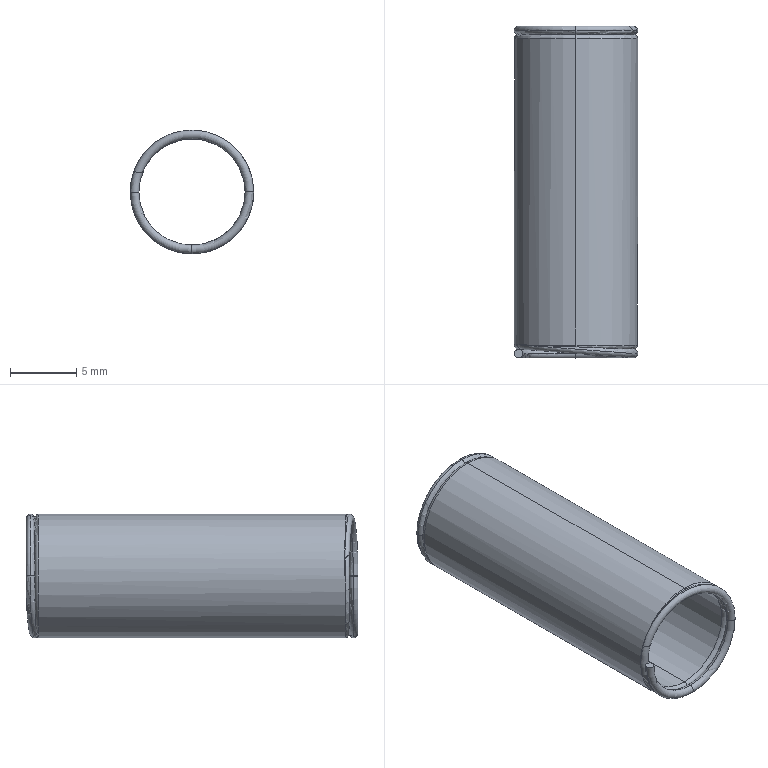Part | STEP file | C-VUR8-25 | 1 solid | 32 faces | box 9.3 x 25 x 9.325 mm | volume 430.371 mm3 | torus 26 | cylinder 4 | plane 2 | commonest cylinder face diameters 8 x2 9.3 x2
STEP:
#1=CARTESIAN_POINT('',(0.,-12.175,-4.65));
#2=VERTEX_POINT('',#1);
#3=CARTESIAN_POINT('',(0.,-12.175,-4.));
#4=VERTEX_POINT('',#3);
#5=CARTESIAN_POINT('',(0.,-12.175,-4.325));
#6=DIRECTION('',(-1.,0.,0.));
#7=DIRECTION('',(0.,0.,1.));
#8=AXIS2_PLACEMENT_3D('',#5,#6,#7);
#9=CIRCLE('',#8,0.325);
#10=EDGE_CURVE('',#2,#4,#9,.T.);
#11=ORIENTED_EDGE('',*,*,#10,.F.);
#12=CARTESIAN_POINT('',(4.65,-12.175,0.));
#13=VERTEX_POINT('',#12);
#14=CARTESIAN_POINT('',(0.,-12.175,0.));
#15=DIRECTION('',(0.,-1.,0.));
#16=DIRECTION('',(0.,0.,-1.));
#17=AXIS2_PLACEMENT_3D('',#14,#15,#16);
#18=CIRCLE('',#17,4.65);
#19=EDGE_CURVE('',#2,#13,#18,.T.);
#20=ORIENTED_EDGE('',*,*,#19,.T.);
#21=CARTESIAN_POINT('',(4.649,-12.2,0.));
#22=VERTEX_POINT('',#21);
#23=CARTESIAN_POINT('',(4.325,-12.175,0.));
#24=DIRECTION('',(0.,0.,1.));
#25=DIRECTION('',(1.,0.,0.));
#26=AXIS2_PLACEMENT_3D('',#23,#24,#25);
#27=CIRCLE('',#26,0.325);
#28=EDGE_CURVE('',#22,#13,#27,.T.);
#29=ORIENTED_EDGE('',*,*,#28,.F.);
#30=CARTESIAN_POINT('',(4.,-12.175,0.));
#31=VERTEX_POINT('',#30);
#32=CARTESIAN_POINT('',(4.325,-12.175,0.));
#33=DIRECTION('',(0.,0.,1.));
#34=DIRECTION('',(1.,0.,0.));
#35=AXIS2_PLACEMENT_3D('',#32,#33,#34);
#36=CIRCLE('',#35,0.325);
#37=EDGE_CURVE('',#31,#22,#36,.T.);
#38=ORIENTED_EDGE('',*,*,#37,.F.);
#39=CARTESIAN_POINT('',(0.,-12.175,0.));
#40=DIRECTION('',(0.,-1.,0.));
#41=DIRECTION('',(0.,0.,-1.));
#42=AXIS2_PLACEMENT_3D('',#39,#40,#41);
#43=CIRCLE('',#42,4.);
#44=EDGE_CURVE('',#4,#31,#43,.T.);
#45=ORIENTED_EDGE('',*,*,#44,.F.);
#46=EDGE_LOOP('',(#11,#20,#29,#38,#45));
#47=FACE_OUTER_BOUND('',#46,.T.);
#48=CARTESIAN_POINT('',(0.,-12.175,0.));
#49=DIRECTION('',(0.,-1.,0.));
#50=DIRECTION('',(0.,0.,-1.));
#51=AXIS2_PLACEMENT_3D('',#48,#49,#50);
#52=TOROIDAL_SURFACE('',#51,4.325,0.325);
#53=ADVANCED_FACE('',(#47),#52,.T.);
#54=CARTESIAN_POINT('',(0.,-11.855,-4.268));
#55=VERTEX_POINT('',#54);
#56=CARTESIAN_POINT('',(0.,-12.175,-4.325));
#57=DIRECTION('',(-1.,0.,0.));
#58=DIRECTION('',(0.,0.,1.));
#59=AXIS2_PLACEMENT_3D('',#56,#57,#58);
#60=CIRCLE('',#59,0.325);
#61=EDGE_CURVE('',#4,#55,#60,.T.);
#62=ORIENTED_EDGE('',*,*,#61,.F.);
#63=ORIENTED_EDGE('',*,*,#44,.T.);
#64=CARTESIAN_POINT('',(4.001,-12.15,0.));
#65=VERTEX_POINT('',#64);
#66=CARTESIAN_POINT('',(4.325,-12.175,0.));
#67=DIRECTION('',(0.,0.,1.));
#68=DIRECTION('',(1.,0.,0.));
#69=AXIS2_PLACEMENT_3D('',#66,#67,#68);
#70=CIRCLE('',#69,0.325);
#71=EDGE_CURVE('',#65,#31,#70,.T.);
#72=ORIENTED_EDGE('',*,*,#71,.F.);
#73=CARTESIAN_POINT('',(4.268,-11.855,0.));
#74=VERTEX_POINT('',#73);
#75=CARTESIAN_POINT('',(4.325,-12.175,0.));
#76=DIRECTION('',(0.,0.,1.));
#77=DIRECTION('',(1.,0.,0.));
#78=AXIS2_PLACEMENT_3D('',#75,#76,#77);
#79=CIRCLE('',#78,0.325);
#80=EDGE_CURVE('',#74,#65,#79,.T.);
#81=ORIENTED_EDGE('',*,*,#80,.F.);
#82=CARTESIAN_POINT('',(0.,-11.855,0.));
#83=DIRECTION('',(0.,1.,0.));
#84=DIRECTION('',(0.,0.,1.));
#85=AXIS2_PLACEMENT_3D('',#82,#83,#84);
#86=CIRCLE('',#85,4.268);
#87=EDGE_CURVE('',#74,#55,#86,.T.);
#88=ORIENTED_EDGE('',*,*,#87,.T.);
#89=EDGE_LOOP('',(#62,#63,#72,#81,#88));
#90=FACE_OUTER_BOUND('',#89,.T.);
#91=CARTESIAN_POINT('',(0.,-12.175,0.));
#92=DIRECTION('',(0.,-1.,0.));
#93=DIRECTION('',(0.,0.,-1.));
#94=AXIS2_PLACEMENT_3D('',#91,#92,#93);
#95=TOROIDAL_SURFACE('',#94,4.325,0.325);
#96=ADVANCED_FACE('',(#90),#95,.T.);
#97=CARTESIAN_POINT('',(0.,12.175,4.65));
#98=VERTEX_POINT('',#97);
#99=CARTESIAN_POINT('',(0.,12.175,4.));
#100=VERTEX_POINT('',#99);
#101=CARTESIAN_POINT('',(0.,12.175,4.325));
#102=DIRECTION('',(-1.,0.,0.));
#103=DIRECTION('',(0.,0.,1.));
#104=AXIS2_PLACEMENT_3D('',#101,#102,#103);
#105=CIRCLE('',#104,0.325);
#106=EDGE_CURVE('',#98,#100,#105,.T.);
#107=ORIENTED_EDGE('',*,*,#106,.F.);
#108=CARTESIAN_POINT('',(4.65,12.175,0.));
#109=VERTEX_POINT('',#108);
#110=CARTESIAN_POINT('',(0.,12.175,0.));
#111=DIRECTION('',(0.,1.,0.));
#112=DIRECTION('',(0.,0.,1.));
#113=AXIS2_PLACEMENT_3D('',#110,#111,#112);
#114=CIRCLE('',#113,4.65);
#115=EDGE_CURVE('',#98,#109,#114,.T.);
#116=ORIENTED_EDGE('',*,*,#115,.T.);
#117=CARTESIAN_POINT('',(4.,12.175,0.));
#118=VERTEX_POINT('',#117);
#119=CARTESIAN_POINT('',(4.325,12.175,0.));
#120=DIRECTION('',(0.,0.,-1.));
#121=DIRECTION('',(-1.,0.,0.));
#122=AXIS2_PLACEMENT_3D('',#119,#120,#121);
#123=CIRCLE('',#122,0.325);
#124=EDGE_CURVE('',#118,#109,#123,.T.);
#125=ORIENTED_EDGE('',*,*,#124,.F.);
#126=CARTESIAN_POINT('',(0.,12.175,0.));
#127=DIRECTION('',(0.,1.,0.));
#128=DIRECTION('',(0.,0.,1.));
#129=AXIS2_PLACEMENT_3D('',#126,#127,#128);
#130=CIRCLE('',#129,4.);
#131=EDGE_CURVE('',#100,#118,#130,.T.);
#132=ORIENTED_EDGE('',*,*,#131,.F.);
#133=EDGE_LOOP('',(#107,#116,#125,#132));
#134=FACE_OUTER_BOUND('',#133,.T.);
#135=CARTESIAN_POINT('',(0.,12.175,0.));
#136=DIRECTION('',(0.,1.,0.));
#137=DIRECTION('',(0.,0.,1.));
#138=AXIS2_PLACEMENT_3D('',#135,#136,#137);
#139=TOROIDAL_SURFACE('',#138,4.325,0.325);
#140=ADVANCED_FACE('',(#134),#139,.T.);
#141=CARTESIAN_POINT('',(0.,11.855,4.268));
#142=VERTEX_POINT('',#141);
#143=CARTESIAN_POINT('',(0.,12.175,4.325));
#144=DIRECTION('',(-1.,0.,0.));
#145=DIRECTION('',(0.,0.,1.));
#146=AXIS2_PLACEMENT_3D('',#143,#144,#145);
#147=CIRCLE('',#146,0.325);
#148=EDGE_CURVE('',#100,#142,#147,.T.);
#149=ORIENTED_EDGE('',*,*,#148,.F.);
#150=ORIENTED_EDGE('',*,*,#131,.T.);
#151=CARTESIAN_POINT('',(4.268,11.855,0.));
#152=VERTEX_POINT('',#151);
#153=CARTESIAN_POINT('',(4.325,12.175,0.));
#154=DIRECTION('',(0.,0.,-1.));
#155=DIRECTION('',(-1.,0.,0.));
#156=AXIS2_PLACEMENT_3D('',#153,#154,#155);
#157=CIRCLE('',#156,0.325);
#158=EDGE_CURVE('',#152,#118,#157,.T.);
#159=ORIENTED_EDGE('',*,*,#158,.F.);
#160=CARTESIAN_POINT('',(0.,11.855,0.));
#161=DIRECTION('',(0.,-1.,0.));
#162=DIRECTION('',(0.,0.,-1.));
#163=AXIS2_PLACEMENT_3D('',#160,#161,#162);
#164=CIRCLE('',#163,4.268);
#165=EDGE_CURVE('',#152,#142,#164,.T.);
#166=ORIENTED_EDGE('',*,*,#165,.T.);
#167=EDGE_LOOP('',(#149,#150,#159,#166));
#168=FACE_OUTER_BOUND('',#167,.T.);
#169=CARTESIAN_POINT('',(0.,12.175,0.));
#170=DIRECTION('',(0.,1.,0.));
#171=DIRECTION('',(0.,0.,1.));
#172=AXIS2_PLACEMENT_3D('',#169,#170,#171);
#173=TOROIDAL_SURFACE('',#172,4.325,0.325);
#174=ADVANCED_FACE('',(#168),#173,.T.);
#175=CARTESIAN_POINT('',(4.65,11.515,0.));
#176=VERTEX_POINT('',#175);
#177=CARTESIAN_POINT('',(4.484,11.503,-1.23));
#178=VERTEX_POINT('',#177);
#179=CARTESIAN_POINT('',(4.65,11.515,0.));
#180=CARTESIAN_POINT('',(4.65,11.511,-0.2071));
#181=CARTESIAN_POINT('',(4.636,11.508,-0.4155));
#182=CARTESIAN_POINT('',(4.581,11.504,-0.8261));
#183=CARTESIAN_POINT('',(4.539,11.503,-1.029));
#184=CARTESIAN_POINT('',(4.484,11.503,-1.23));
#185=B_SPLINE_CURVE_WITH_KNOTS('',3,(#179,#180,#181,#182,#183,#184),.UNSPECIFIED.,.F.,.F.,(4,2,4),(-0.0001859,0.0004355,0.001057),.UNSPECIFIED.);
#186=EDGE_CURVE('',#176,#178,#185,.T.);
#187=ORIENTED_EDGE('',*,*,#186,.T.);
#188=CARTESIAN_POINT('',(-4.649,12.2,0.));
#189=VERTEX_POINT('',#188);
#190=CARTESIAN_POINT('',(0.,11.845,0.));
#191=DIRECTION('',(0.07608,0.9971,0.));
#192=DIRECTION('',(-0.9971,0.07608,0.));
#193=AXIS2_PLACEMENT_3D('',#190,#191,#192);
#194=CIRCLE('',#193,4.663);
#195=EDGE_CURVE('',#178,#189,#194,.T.);
#196=ORIENTED_EDGE('',*,*,#195,.T.);
#197=CARTESIAN_POINT('',(-4.,12.175,0.));
#198=VERTEX_POINT('',#197);
#199=CARTESIAN_POINT('',(-4.325,12.175,0.));
#200=DIRECTION('',(0.,0.,1.));
#201=DIRECTION('',(1.,0.,0.));
#202=AXIS2_PLACEMENT_3D('',#199,#200,#201);
#203=CIRCLE('',#202,0.325);
#204=EDGE_CURVE('',#198,#189,#203,.T.);
#205=ORIENTED_EDGE('',*,*,#204,.F.);
#206=CARTESIAN_POINT('',(-4.001,12.15,0.));
#207=VERTEX_POINT('',#206);
#208=CARTESIAN_POINT('',(-4.325,12.175,0.));
#209=DIRECTION('',(0.,0.,1.));
#210=DIRECTION('',(1.,0.,0.));
#211=AXIS2_PLACEMENT_3D('',#208,#209,#210);
#212=CIRCLE('',#211,0.325);
#213=EDGE_CURVE('',#207,#198,#212,.T.);
#214=ORIENTED_EDGE('',*,*,#213,.F.);
#215=CARTESIAN_POINT('',(3.371,11.588,-2.162));
#216=VERTEX_POINT('',#215);
#217=CARTESIAN_POINT('',(0.,11.845,0.));
#218=DIRECTION('',(0.07608,0.9971,0.));
#219=DIRECTION('',(-0.9971,0.07608,0.));
#220=AXIS2_PLACEMENT_3D('',#217,#218,#219);
#221=CIRCLE('',#220,4.013);
#222=EDGE_CURVE('',#216,#207,#221,.T.);
#223=ORIENTED_EDGE('',*,*,#222,.F.);
#224=CARTESIAN_POINT('',(4.583,11.535,-0.7869));
#225=VERTEX_POINT('',#224);
#226=CARTESIAN_POINT('',(3.371,11.588,-2.162));
#227=CARTESIAN_POINT('',(3.422,11.588,-2.082));
#228=CARTESIAN_POINT('',(3.471,11.588,-1.999));
#229=CARTESIAN_POINT('',(3.564,11.594,-1.831));
#230=CARTESIAN_POINT('',(3.607,11.597,-1.745));
#231=CARTESIAN_POINT('',(3.671,11.619,-1.617));
#232=CARTESIAN_POINT('',(3.692,11.629,-1.574));
#233=CARTESIAN_POINT('',(3.739,11.67,-1.501));
#234=CARTESIAN_POINT('',(3.766,11.705,-1.475));
#235=CARTESIAN_POINT('',(3.832,11.772,-1.454));
#236=CARTESIAN_POINT('',(3.871,11.803,-1.455));
#237=CARTESIAN_POINT('',(3.957,11.846,-1.464));
#238=CARTESIAN_POINT('',(4.004,11.858,-1.472));
#239=CARTESIAN_POINT('',(4.098,11.862,-1.489));
#240=CARTESIAN_POINT('',(4.146,11.853,-1.498));
#241=CARTESIAN_POINT('',(4.234,11.816,-1.51));
#242=CARTESIAN_POINT('',(4.275,11.788,-1.513));
#243=CARTESIAN_POINT('',(4.343,11.72,-1.503));
#244=CARTESIAN_POINT('',(4.371,11.681,-1.489));
#245=CARTESIAN_POINT('',(4.415,11.62,-1.428));
#246=CARTESIAN_POINT('',(4.432,11.601,-1.386));
#247=CARTESIAN_POINT('',(4.478,11.563,-1.254));
#248=CARTESIAN_POINT('',(4.503,11.555,-1.161));
#249=CARTESIAN_POINT('',(4.548,11.542,-0.9752));
#250=CARTESIAN_POINT('',(4.567,11.538,-0.8814));
#251=CARTESIAN_POINT('',(4.583,11.535,-0.7869));
#252=B_SPLINE_CURVE_WITH_KNOTS('',3,(#226,#227,#228,#229,#230,#231,#232,#233,#234,#235,#236,#237,#238,#239,#240,#241,#242,#243,#244,#245,#246,#247,#248,#249,#250,#251),.UNSPECIFIED.,.F.,.F.,(4,2,2,2,2,2,2,2,2,2,2,2,4),(0.01059,0.01088,0.01117,0.01131,0.01146,0.0116,0.01175,0.01189,0.01203,0.01218,0.01232,0.01261,0.0129),.UNSPECIFIED.);
#253=EDGE_CURVE('',#216,#225,#252,.T.);
#254=ORIENTED_EDGE('',*,*,#253,.T.);
#255=CARTESIAN_POINT('',(4.583,11.535,-0.7869));
#256=CARTESIAN_POINT('',(4.628,11.527,-0.5268));
#257=CARTESIAN_POINT('',(4.65,11.52,-0.2635));
#258=CARTESIAN_POINT('',(4.65,11.515,0.));
#259=B_SPLINE_CURVE_WITH_KNOTS('',3,(#255,#256,#257,#258),.UNSPECIFIED.,.F.,.F.,(4,4),(-0.0001859,0.0006046),.UNSPECIFIED.);
#260=EDGE_CURVE('',#225,#176,#259,.T.);
#261=ORIENTED_EDGE('',*,*,#260,.T.);
#262=EDGE_LOOP('',(#187,#196,#205,#214,#223,#254,#261));
#263=FACE_OUTER_BOUND('',#262,.T.);
#264=CARTESIAN_POINT('',(0.,11.845,0.));
#265=DIRECTION('',(0.07608,0.9971,0.));
#266=DIRECTION('',(-0.9971,0.07608,0.));
#267=AXIS2_PLACEMENT_3D('',#264,#265,#266);
#268=TOROIDAL_SURFACE('',#267,4.338,0.325);
#269=ADVANCED_FACE('',(#263),#268,.T.);
#270=CARTESIAN_POINT('',(0.,11.701,-4.046));
#271=VERTEX_POINT('',#270);
#272=CARTESIAN_POINT('',(0.,11.701,-4.046));
#273=CARTESIAN_POINT('',(0.1676,11.695,-4.042));
#274=CARTESIAN_POINT('',(0.3369,11.689,-4.028));
#275=CARTESIAN_POINT('',(0.6686,11.677,-3.98));
#276=CARTESIAN_POINT('',(0.8319,11.671,-3.946));
#277=CARTESIAN_POINT('',(1.154,11.659,-3.859));
#278=CARTESIAN_POINT('',(1.312,11.653,-3.806));
#279=CARTESIAN_POINT('',(1.623,11.642,-3.679));
#280=CARTESIAN_POINT('',(1.776,11.636,-3.606));
#281=CARTESIAN_POINT('',(2.214,11.62,-3.361));
#282=CARTESIAN_POINT('',(2.484,11.611,-3.165));
#283=CARTESIAN_POINT('',(2.976,11.595,-2.702));
#284=CARTESIAN_POINT('',(3.19,11.588,-2.444));
#285=CARTESIAN_POINT('',(3.371,11.588,-2.162));
#286=B_SPLINE_CURVE_WITH_KNOTS('',3,(#272,#273,#274,#275,#276,#277,#278,#279,#280,#281,#282,#283,#284,#285),.UNSPECIFIED.,.F.,.F.,(4,2,2,2,2,2,4),(0.006551,0.007056,0.007562,0.008067,0.008573,0.009584,0.01059),.UNSPECIFIED.);
#287=EDGE_CURVE('',#271,#216,#286,.T.);
#288=ORIENTED_EDGE('',*,*,#287,.T.);
#289=ORIENTED_EDGE('',*,*,#222,.T.);
#290=CARTESIAN_POINT('',(-4.268,11.855,0.));
#291=VERTEX_POINT('',#290);
#292=CARTESIAN_POINT('',(-4.325,12.175,0.));
#293=DIRECTION('',(0.,0.,1.));
#294=DIRECTION('',(1.,0.,0.));
#295=AXIS2_PLACEMENT_3D('',#292,#293,#294);
#296=CIRCLE('',#295,0.325);
#297=EDGE_CURVE('',#291,#207,#296,.T.);
#298=ORIENTED_EDGE('',*,*,#297,.F.);
#299=CARTESIAN_POINT('',(-4.268,11.855,0.));
#300=CARTESIAN_POINT('',(-4.268,11.855,-1.096));
#301=CARTESIAN_POINT('',(-3.752,11.838,-2.168));
#302=CARTESIAN_POINT('',(-2.765,11.803,-3.093));
#303=CARTESIAN_POINT('',(-2.548,11.795,-3.261));
#304=CARTESIAN_POINT('',(-2.087,11.778,-3.55));
#305=CARTESIAN_POINT('',(-1.845,11.769,-3.671));
#306=CARTESIAN_POINT('',(-1.34,11.751,-3.865));
#307=CARTESIAN_POINT('',(-1.074,11.741,-3.938));
#308=CARTESIAN_POINT('',(-0.5406,11.721,-4.031));
#309=CARTESIAN_POINT('',(-0.2715,11.711,-4.052));
#310=CARTESIAN_POINT('',(0.,11.701,-4.046));
#311=B_SPLINE_CURVE_WITH_KNOTS('',3,(#299,#300,#301,#302,#303,#304,#305,#306,#307,#308,#309,#310),.UNSPECIFIED.,.F.,.F.,(4,2,2,2,2,4),(0.,0.003275,0.004094,0.004913,0.005732,0.006551),.UNSPECIFIED.);
#312=EDGE_CURVE('',#291,#271,#311,.T.);
#313=ORIENTED_EDGE('',*,*,#312,.T.);
#314=EDGE_LOOP('',(#288,#289,#298,#313));
#315=FACE_OUTER_BOUND('',#314,.T.);
#316=CARTESIAN_POINT('',(0.,11.845,0.));
#317=DIRECTION('',(0.07608,0.9971,0.));
#318=DIRECTION('',(-0.9971,0.07608,0.));
#319=AXIS2_PLACEMENT_3D('',#316,#317,#318);
#320=TOROIDAL_SURFACE('',#319,4.338,0.325);
#321=ADVANCED_FACE('',(#315),#320,.T.);
#322=ORIENTED_EDGE('',*,*,#71,.T.);
#323=ORIENTED_EDGE('',*,*,#37,.T.);
#324=CARTESIAN_POINT('',(-4.484,-11.503,1.23));
#325=VERTEX_POINT('',#324);
#326=CARTESIAN_POINT('',(0.,-11.845,0.));
#327=DIRECTION('',(-0.07608,-0.9971,0.));
#328=DIRECTION('',(0.9971,-0.07608,0.));
#329=AXIS2_PLACEMENT_3D('',#326,#327,#328);
#330=CIRCLE('',#329,4.663);
#331=EDGE_CURVE('',#22,#325,#330,.T.);
#332=ORIENTED_EDGE('',*,*,#331,.T.);
#333=CARTESIAN_POINT('',(-4.65,-11.515,0.));
#334=VERTEX_POINT('',#333);
#335=CARTESIAN_POINT('',(-4.484,-11.503,1.23));
#336=CARTESIAN_POINT('',(-4.594,-11.503,0.8286));
#337=CARTESIAN_POINT('',(-4.65,-11.508,0.416));
#338=CARTESIAN_POINT('',(-4.65,-11.515,0.));
#339=B_SPLINE_CURVE_WITH_KNOTS('',3,(#335,#336,#337,#338),.UNSPECIFIED.,.F.,.F.,(4,4),(0.002037,0.003284),.UNSPECIFIED.);
#340=EDGE_CURVE('',#325,#334,#339,.T.);
#341=ORIENTED_EDGE('',*,*,#340,.T.);
#342=CARTESIAN_POINT('',(-4.583,-11.535,0.7869));
#343=VERTEX_POINT('',#342);
#344=CARTESIAN_POINT('',(-4.65,-11.515,0.));
#345=CARTESIAN_POINT('',(-4.65,-11.52,0.2635));
#346=CARTESIAN_POINT('',(-4.628,-11.527,0.5268));
#347=CARTESIAN_POINT('',(-4.583,-11.535,0.7869));
#348=B_SPLINE_CURVE_WITH_KNOTS('',3,(#344,#345,#346,#347),.UNSPECIFIED.,.F.,.F.,(4,4),(-0.0001859,0.0006046),.UNSPECIFIED.);
#349=EDGE_CURVE('',#334,#343,#348,.T.);
#350=ORIENTED_EDGE('',*,*,#349,.T.);
#351=CARTESIAN_POINT('',(-3.371,-11.588,2.162));
#352=VERTEX_POINT('',#351);
#353=CARTESIAN_POINT('',(-4.583,-11.535,0.7869));
#354=CARTESIAN_POINT('',(-4.567,-11.538,0.8818));
#355=CARTESIAN_POINT('',(-4.547,-11.542,0.9761));
#356=CARTESIAN_POINT('',(-4.503,-11.555,1.163));
#357=CARTESIAN_POINT('',(-4.478,-11.563,1.257));
#358=CARTESIAN_POINT('',(-4.431,-11.602,1.388));
#359=CARTESIAN_POINT('',(-4.414,-11.621,1.431));
#360=CARTESIAN_POINT('',(-4.37,-11.682,1.49));
#361=CARTESIAN_POINT('',(-4.341,-11.722,1.504));
#362=CARTESIAN_POINT('',(-4.273,-11.789,1.513));
#363=CARTESIAN_POINT('',(-4.232,-11.817,1.51));
#364=CARTESIAN_POINT('',(-4.143,-11.853,1.497));
#365=CARTESIAN_POINT('',(-4.096,-11.862,1.489));
#366=CARTESIAN_POINT('',(-4.001,-11.858,1.472));
#367=CARTESIAN_POINT('',(-3.954,-11.845,1.464));
#368=CARTESIAN_POINT('',(-3.869,-11.802,1.455));
#369=CARTESIAN_POINT('',(-3.831,-11.771,1.454));
#370=CARTESIAN_POINT('',(-3.765,-11.704,1.475));
#371=CARTESIAN_POINT('',(-3.738,-11.669,1.502));
#372=CARTESIAN_POINT('',(-3.691,-11.629,1.576));
#373=CARTESIAN_POINT('',(-3.67,-11.619,1.619));
#374=CARTESIAN_POINT('',(-3.607,-11.597,1.746));
#375=CARTESIAN_POINT('',(-3.563,-11.594,1.832));
#376=CARTESIAN_POINT('',(-3.471,-11.588,1.999));
#377=CARTESIAN_POINT('',(-3.422,-11.588,2.082));
#378=CARTESIAN_POINT('',(-3.371,-11.588,2.162));
#379=B_SPLINE_CURVE_WITH_KNOTS('',3,(#353,#354,#355,#356,#357,#358,#359,#360,#361,#362,#363,#364,#365,#366,#367,#368,#369,#370,#371,#372,#373,#374,#375,#376,#377,#378),.UNSPECIFIED.,.F.,.F.,(4,2,2,2,2,2,2,2,2,2,2,2,4),(0.,0.0002887,0.0005774,0.0007218,0.0008661,0.00101,0.001155,0.001299,0.001444,0.001588,0.001732,0.002021,0.00231),.UNSPECIFIED.);
#380=EDGE_CURVE('',#343,#352,#379,.T.);
#381=ORIENTED_EDGE('',*,*,#380,.T.);
#382=CARTESIAN_POINT('',(0.,-11.845,0.));
#383=DIRECTION('',(-0.07608,-0.9971,0.));
#384=DIRECTION('',(0.9971,-0.07608,0.));
#385=AXIS2_PLACEMENT_3D('',#382,#383,#384);
#386=CIRCLE('',#385,4.013);
#387=EDGE_CURVE('',#65,#352,#386,.T.);
#388=ORIENTED_EDGE('',*,*,#387,.F.);
#389=EDGE_LOOP('',(#322,#323,#332,#341,#350,#381,#388));
#390=FACE_OUTER_BOUND('',#389,.T.);
#391=CARTESIAN_POINT('',(0.,-11.845,0.));
#392=DIRECTION('',(-0.07608,-0.9971,0.));
#393=DIRECTION('',(0.9971,-0.07608,0.));
#394=AXIS2_PLACEMENT_3D('',#391,#392,#393);
#395=TOROIDAL_SURFACE('',#394,4.338,0.325);
#396=ADVANCED_FACE('',(#390),#395,.T.);
#397=ORIENTED_EDGE('',*,*,#80,.T.);
#398=ORIENTED_EDGE('',*,*,#387,.T.);
#399=CARTESIAN_POINT('',(0.,-11.701,4.046));
#400=VERTEX_POINT('',#399);
#401=CARTESIAN_POINT('',(-3.371,-11.588,2.162));
#402=CARTESIAN_POINT('',(-3.189,-11.588,2.445));
#403=CARTESIAN_POINT('',(-2.971,-11.595,2.707));
#404=CARTESIAN_POINT('',(-2.607,-11.607,3.049));
#405=CARTESIAN_POINT('',(-2.478,-11.611,3.156));
#406=CARTESIAN_POINT('',(-2.208,-11.621,3.353));
#407=CARTESIAN_POINT('',(-2.065,-11.626,3.445));
#408=CARTESIAN_POINT('',(-1.625,-11.642,3.69));
#409=CARTESIAN_POINT('',(-1.316,-11.653,3.815));
#410=CARTESIAN_POINT('',(-0.8299,-11.671,3.947));
#411=CARTESIAN_POINT('',(-0.6639,-11.677,3.981));
#412=CARTESIAN_POINT('',(-0.3328,-11.689,4.029));
#413=CARTESIAN_POINT('',(-0.1667,-11.695,4.042));
#414=CARTESIAN_POINT('',(0.,-11.701,4.046));
#415=B_SPLINE_CURVE_WITH_KNOTS('',3,(#401,#402,#403,#404,#405,#406,#407,#408,#409,#410,#411,#412,#413,#414),.UNSPECIFIED.,.F.,.F.,(4,2,2,2,2,2,4),(0.00231,0.003326,0.003834,0.004342,0.005359,0.005867,0.006375),.UNSPECIFIED.);
#416=EDGE_CURVE('',#352,#400,#415,.T.);
#417=ORIENTED_EDGE('',*,*,#416,.T.);
#418=CARTESIAN_POINT('',(0.,-11.701,4.046));
#419=CARTESIAN_POINT('',(0.2695,-11.711,4.052));
#420=CARTESIAN_POINT('',(0.5434,-11.721,4.031));
#421=CARTESIAN_POINT('',(1.077,-11.741,3.938));
#422=CARTESIAN_POINT('',(1.337,-11.751,3.866));
#423=CARTESIAN_POINT('',(1.842,-11.769,3.672));
#424=CARTESIAN_POINT('',(2.088,-11.778,3.549));
#425=CARTESIAN_POINT('',(2.549,-11.795,3.26));
#426=CARTESIAN_POINT('',(2.766,-11.803,3.093));
#427=CARTESIAN_POINT('',(3.363,-11.824,2.532));
#428=CARTESIAN_POINT('',(3.687,-11.835,2.081));
#429=CARTESIAN_POINT('',(4.139,-11.851,1.089));
#430=CARTESIAN_POINT('',(4.268,-11.855,0.5469));
#431=CARTESIAN_POINT('',(4.268,-11.855,0.));
#432=B_SPLINE_CURVE_WITH_KNOTS('',3,(#418,#419,#420,#421,#422,#423,#424,#425,#426,#427,#428,#429,#430,#431),.UNSPECIFIED.,.F.,.F.,(4,2,2,2,2,2,4),(0.006375,0.007196,0.008018,0.00884,0.009661,0.0113,0.01295),.UNSPECIFIED.);
#433=EDGE_CURVE('',#400,#74,#432,.T.);
#434=ORIENTED_EDGE('',*,*,#433,.T.);
#435=EDGE_LOOP('',(#397,#398,#417,#434));
#436=FACE_OUTER_BOUND('',#435,.T.);
#437=CARTESIAN_POINT('',(0.,-11.845,0.));
#438=DIRECTION('',(-0.07608,-0.9971,0.));
#439=DIRECTION('',(0.9971,-0.07608,0.));
#440=AXIS2_PLACEMENT_3D('',#437,#438,#439);
#441=TOROIDAL_SURFACE('',#440,4.338,0.325);
#442=ADVANCED_FACE('',(#436),#441,.T.);
#443=ORIENTED_EDGE('',*,*,#204,.T.);
#444=CARTESIAN_POINT('',(-4.65,12.175,0.));
#445=VERTEX_POINT('',#444);
#446=CARTESIAN_POINT('',(-4.325,12.175,0.));
#447=DIRECTION('',(0.,0.,1.));
#448=DIRECTION('',(1.,0.,0.));
#449=AXIS2_PLACEMENT_3D('',#446,#447,#448);
#450=CIRCLE('',#449,0.325);
#451=EDGE_CURVE('',#189,#445,#450,.T.);
#452=ORIENTED_EDGE('',*,*,#451,.T.);
#453=CARTESIAN_POINT('',(0.,12.175,0.));
#454=DIRECTION('',(0.,1.,0.));
#455=DIRECTION('',(0.,0.,1.));
#456=AXIS2_PLACEMENT_3D('',#453,#454,#455);
#457=CIRCLE('',#456,4.65);
#458=EDGE_CURVE('',#445,#98,#457,.T.);
#459=ORIENTED_EDGE('',*,*,#458,.T.);
#460=ORIENTED_EDGE('',*,*,#106,.T.);
#461=CARTESIAN_POINT('',(0.,12.175,0.));
#462=DIRECTION('',(0.,1.,0.));
#463=DIRECTION('',(0.,0.,1.));
#464=AXIS2_PLACEMENT_3D('',#461,#462,#463);
#465=CIRCLE('',#464,4.);
#466=EDGE_CURVE('',#198,#100,#465,.T.);
#467=ORIENTED_EDGE('',*,*,#466,.F.);
#468=EDGE_LOOP('',(#443,#452,#459,#460,#467));
#469=FACE_OUTER_BOUND('',#468,.T.);
#470=CARTESIAN_POINT('',(0.,12.175,0.));
#471=DIRECTION('',(0.,1.,0.));
#472=DIRECTION('',(0.,0.,1.));
#473=AXIS2_PLACEMENT_3D('',#470,#471,#472);
#474=TOROIDAL_SURFACE('',#473,4.325,0.325);
#475=ADVANCED_FACE('',(#469),#474,.T.);
#476=ORIENTED_EDGE('',*,*,#297,.T.);
#477=ORIENTED_EDGE('',*,*,#213,.T.);
#478=ORIENTED_EDGE('',*,*,#466,.T.);
#479=ORIENTED_EDGE('',*,*,#148,.T.);
#480=CARTESIAN_POINT('',(0.,11.855,0.));
#481=DIRECTION('',(0.,-1.,0.));
#482=DIRECTION('',(0.,0.,-1.));
#483=AXIS2_PLACEMENT_3D('',#480,#481,#482);
#484=CIRCLE('',#483,4.268);
#485=EDGE_CURVE('',#142,#291,#484,.T.);
#486=ORIENTED_EDGE('',*,*,#485,.T.);
#487=EDGE_LOOP('',(#476,#477,#478,#479,#486));
#488=FACE_OUTER_BOUND('',#487,.T.);
#489=CARTESIAN_POINT('',(0.,12.175,0.));
#490=DIRECTION('',(0.,1.,0.));
#491=DIRECTION('',(0.,0.,1.));
#492=AXIS2_PLACEMENT_3D('',#489,#490,#491);
#493=TOROIDAL_SURFACE('',#492,4.325,0.325);
#494=ADVANCED_FACE('',(#488),#493,.T.);
#495=CARTESIAN_POINT('',(-4.,-12.175,0.));
#496=VERTEX_POINT('',#495);
#497=CARTESIAN_POINT('',(-4.65,-12.175,0.));
#498=VERTEX_POINT('',#497);
#499=CARTESIAN_POINT('',(-4.325,-12.175,0.));
#500=DIRECTION('',(0.,0.,-1.));
#501=DIRECTION('',(-1.,0.,0.));
#502=AXIS2_PLACEMENT_3D('',#499,#500,#501);
#503=CIRCLE('',#502,0.325);
#504=EDGE_CURVE('',#496,#498,#503,.T.);
#505=ORIENTED_EDGE('',*,*,#504,.T.);
#506=CARTESIAN_POINT('',(0.,-12.175,0.));
#507=DIRECTION('',(0.,-1.,0.));
#508=DIRECTION('',(0.,0.,-1.));
#509=AXIS2_PLACEMENT_3D('',#506,#507,#508);
#510=CIRCLE('',#509,4.65);
#511=EDGE_CURVE('',#498,#2,#510,.T.);
#512=ORIENTED_EDGE('',*,*,#511,.T.);
#513=ORIENTED_EDGE('',*,*,#10,.T.);
#514=CARTESIAN_POINT('',(0.,-12.175,0.));
#515=DIRECTION('',(0.,-1.,0.));
#516=DIRECTION('',(0.,0.,-1.));
#517=AXIS2_PLACEMENT_3D('',#514,#515,#516);
#518=CIRCLE('',#517,4.);
#519=EDGE_CURVE('',#496,#4,#518,.T.);
#520=ORIENTED_EDGE('',*,*,#519,.F.);
#521=EDGE_LOOP('',(#505,#512,#513,#520));
#522=FACE_OUTER_BOUND('',#521,.T.);
#523=CARTESIAN_POINT('',(0.,-12.175,0.));
#524=DIRECTION('',(0.,-1.,0.));
#525=DIRECTION('',(0.,0.,-1.));
#526=AXIS2_PLACEMENT_3D('',#523,#524,#525);
#527=TOROIDAL_SURFACE('',#526,4.325,0.325);
#528=ADVANCED_FACE('',(#522),#527,.T.);
#529=CARTESIAN_POINT('',(-4.268,-11.855,0.));
#530=VERTEX_POINT('',#529);
#531=CARTESIAN_POINT('',(-4.325,-12.175,0.));
#532=DIRECTION('',(0.,0.,-1.));
#533=DIRECTION('',(-1.,0.,0.));
#534=AXIS2_PLACEMENT_3D('',#531,#532,#533);
#535=CIRCLE('',#534,0.325);
#536=EDGE_CURVE('',#530,#496,#535,.T.);
#537=ORIENTED_EDGE('',*,*,#536,.T.);
#538=ORIENTED_EDGE('',*,*,#519,.T.);
#539=ORIENTED_EDGE('',*,*,#61,.T.);
#540=CARTESIAN_POINT('',(0.,-11.855,0.));
#541=DIRECTION('',(0.,1.,0.));
#542=DIRECTION('',(0.,0.,1.));
#543=AXIS2_PLACEMENT_3D('',#540,#541,#542);
#544=CIRCLE('',#543,4.268);
#545=EDGE_CURVE('',#55,#530,#544,.T.);
#546=ORIENTED_EDGE('',*,*,#545,.T.);
#547=EDGE_LOOP('',(#537,#538,#539,#546));
#548=FACE_OUTER_BOUND('',#547,.T.);
#549=CARTESIAN_POINT('',(0.,-12.175,0.));
#550=DIRECTION('',(0.,-1.,0.));
#551=DIRECTION('',(0.,0.,-1.));
#552=AXIS2_PLACEMENT_3D('',#549,#550,#551);
#553=TOROIDAL_SURFACE('',#552,4.325,0.325);
#554=ADVANCED_FACE('',(#548),#553,.T.);
#555=ORIENTED_EDGE('',*,*,#511,.F.);
#556=CARTESIAN_POINT('',(-4.382,-11.855,0.));
#557=VERTEX_POINT('',#556);
#558=CARTESIAN_POINT('',(-4.325,-12.175,0.));
#559=DIRECTION('',(0.,0.,-1.));
#560=DIRECTION('',(-1.,0.,0.));
#561=AXIS2_PLACEMENT_3D('',#558,#559,#560);
#562=CIRCLE('',#561,0.325);
#563=EDGE_CURVE('',#498,#557,#562,.T.);
#564=ORIENTED_EDGE('',*,*,#563,.T.);
#565=CARTESIAN_POINT('',(0.,-11.855,-4.382));
#566=VERTEX_POINT('',#565);
#567=CARTESIAN_POINT('',(0.,-11.855,0.));
#568=DIRECTION('',(0.,-1.,0.));
#569=DIRECTION('',(0.,0.,-1.));
#570=AXIS2_PLACEMENT_3D('',#567,#568,#569);
#571=CIRCLE('',#570,4.382);
#572=EDGE_CURVE('',#557,#566,#571,.T.);
#573=ORIENTED_EDGE('',*,*,#572,.T.);
#574=CARTESIAN_POINT('',(0.,-12.175,-4.325));
#575=DIRECTION('',(-1.,0.,0.));
#576=DIRECTION('',(0.,0.,1.));
#577=AXIS2_PLACEMENT_3D('',#574,#575,#576);
#578=CIRCLE('',#577,0.325);
#579=EDGE_CURVE('',#566,#2,#578,.T.);
#580=ORIENTED_EDGE('',*,*,#579,.T.);
#581=EDGE_LOOP('',(#555,#564,#573,#580));
#582=FACE_OUTER_BOUND('',#581,.T.);
#583=CARTESIAN_POINT('',(0.,-12.175,0.));
#584=DIRECTION('',(0.,-1.,0.));
#585=DIRECTION('',(0.,0.,-1.));
#586=AXIS2_PLACEMENT_3D('',#583,#584,#585);
#587=TOROIDAL_SURFACE('',#586,4.325,0.325);
#588=ADVANCED_FACE('',(#582),#587,.T.);
#589=CARTESIAN_POINT('',(0.,-11.535,-4.65));
#590=VERTEX_POINT('',#589);
#591=CARTESIAN_POINT('',(0.,-11.535,4.65));
#592=VERTEX_POINT('',#591);
#593=CARTESIAN_POINT('',(0.,-11.535,0.));
#594=DIRECTION('',(0.,-1.,0.));
#595=DIRECTION('',(0.,0.,-1.));
#596=AXIS2_PLACEMENT_3D('',#593,#594,#595);
#597=CIRCLE('',#596,4.65);
#598=EDGE_CURVE('',#590,#592,#597,.T.);
#599=ORIENTED_EDGE('',*,*,#598,.T.);
#600=CARTESIAN_POINT('',(0.,-11.678,4.617));
#601=VERTEX_POINT('',#600);
#602=CARTESIAN_POINT('',(0.,-11.535,4.325));
#603=DIRECTION('',(1.,0.,0.));
#604=DIRECTION('',(0.,0.,-1.));
#605=AXIS2_PLACEMENT_3D('',#602,#603,#604);
#606=CIRCLE('',#605,0.325);
#607=EDGE_CURVE('',#592,#601,#606,.T.);
#608=ORIENTED_EDGE('',*,*,#607,.T.);
#609=CARTESIAN_POINT('',(4.382,-11.855,0.));
#610=VERTEX_POINT('',#609);
#611=CARTESIAN_POINT('',(4.382,-11.855,0.));
#612=CARTESIAN_POINT('',(4.382,-11.855,0.2971));
#613=CARTESIAN_POINT('',(4.358,-11.854,0.5946));
#614=CARTESIAN_POINT('',(4.259,-11.849,1.177));
#615=CARTESIAN_POINT('',(4.182,-11.846,1.461));
#616=CARTESIAN_POINT('',(3.974,-11.837,2.015));
#617=CARTESIAN_POINT('',(3.842,-11.831,2.282));
#618=CARTESIAN_POINT('',(3.532,-11.819,2.778));
#619=CARTESIAN_POINT('',(3.353,-11.811,3.011));
#620=CARTESIAN_POINT('',(2.945,-11.795,3.443));
#621=CARTESIAN_POINT('',(2.722,-11.786,3.635));
#622=CARTESIAN_POINT('',(2.243,-11.767,3.973));
#623=CARTESIAN_POINT('',(1.983,-11.756,4.12));
#624=CARTESIAN_POINT('',(1.444,-11.735,4.358));
#625=CARTESIAN_POINT('',(1.165,-11.724,4.449));
#626=CARTESIAN_POINT('',(0.5906,-11.701,4.576));
#627=CARTESIAN_POINT('',(0.2933,-11.69,4.611));
#628=CARTESIAN_POINT('',(0.,-11.678,4.617));
#629=B_SPLINE_CURVE_WITH_KNOTS('',3,(#611,#612,#613,#614,#615,#616,#617,#618,#619,#620,#621,#622,#623,#624,#625,#626,#627,#628),.UNSPECIFIED.,.F.,.F.,(4,2,2,2,2,2,2,2,4),(0.,0.0008898,0.00178,0.002669,0.003559,0.004449,0.005339,0.006229,0.007119),.UNSPECIFIED.);
#630=EDGE_CURVE('',#610,#601,#629,.T.);
#631=ORIENTED_EDGE('',*,*,#630,.F.);
#632=CARTESIAN_POINT('',(0.,-11.855,0.));
#633=DIRECTION('',(0.,-1.,0.));
#634=DIRECTION('',(0.,0.,-1.));
#635=AXIS2_PLACEMENT_3D('',#632,#633,#634);
#636=CIRCLE('',#635,4.382);
#637=EDGE_CURVE('',#566,#610,#636,.T.);
#638=ORIENTED_EDGE('',*,*,#637,.F.);
#639=CARTESIAN_POINT('',(0.,-11.535,-4.325));
#640=DIRECTION('',(-1.,0.,0.));
#641=DIRECTION('',(0.,0.,1.));
#642=AXIS2_PLACEMENT_3D('',#639,#640,#641);
#643=CIRCLE('',#642,0.325);
#644=EDGE_CURVE('',#590,#566,#643,.T.);
#645=ORIENTED_EDGE('',*,*,#644,.F.);
#646=EDGE_LOOP('',(#599,#608,#631,#638,#645));
#647=FACE_OUTER_BOUND('',#646,.T.);
#648=CARTESIAN_POINT('',(0.,-11.535,0.));
#649=DIRECTION('',(0.,-1.,0.));
#650=DIRECTION('',(0.,0.,-1.));
#651=AXIS2_PLACEMENT_3D('',#648,#649,#650);
#652=TOROIDAL_SURFACE('',#651,4.325,0.325);
#653=ADVANCED_FACE('',(#647),#652,.T.);
#654=ORIENTED_EDGE('',*,*,#433,.F.);
#655=CARTESIAN_POINT('',(0.,-11.535,4.));
#656=VERTEX_POINT('',#655);
#657=CARTESIAN_POINT('',(0.,-11.535,4.325));
#658=DIRECTION('',(1.,0.,0.));
#659=DIRECTION('',(0.,0.,-1.));
#660=AXIS2_PLACEMENT_3D('',#657,#658,#659);
#661=CIRCLE('',#660,0.325);
#662=EDGE_CURVE('',#400,#656,#661,.T.);
#663=ORIENTED_EDGE('',*,*,#662,.T.);
#664=CARTESIAN_POINT('',(0.,-11.535,-4.));
#665=VERTEX_POINT('',#664);
#666=CARTESIAN_POINT('',(0.,-11.535,0.));
#667=DIRECTION('',(0.,-1.,0.));
#668=DIRECTION('',(0.,0.,-1.));
#669=AXIS2_PLACEMENT_3D('',#666,#667,#668);
#670=CIRCLE('',#669,4.);
#671=EDGE_CURVE('',#665,#656,#670,.T.);
#672=ORIENTED_EDGE('',*,*,#671,.F.);
#673=CARTESIAN_POINT('',(0.,-11.535,-4.325));
#674=DIRECTION('',(-1.,0.,0.));
#675=DIRECTION('',(0.,0.,1.));
#676=AXIS2_PLACEMENT_3D('',#673,#674,#675);
#677=CIRCLE('',#676,0.325);
#678=EDGE_CURVE('',#55,#665,#677,.T.);
#679=ORIENTED_EDGE('',*,*,#678,.F.);
#680=ORIENTED_EDGE('',*,*,#87,.F.);
#681=EDGE_LOOP('',(#654,#663,#672,#679,#680));
#682=FACE_OUTER_BOUND('',#681,.T.);
#683=CARTESIAN_POINT('',(0.,-11.535,0.));
#684=DIRECTION('',(0.,-1.,0.));
#685=DIRECTION('',(0.,0.,-1.));
#686=AXIS2_PLACEMENT_3D('',#683,#684,#685);
#687=TOROIDAL_SURFACE('',#686,4.325,0.325);
#688=ADVANCED_FACE('',(#682),#687,.T.);
#689=ORIENTED_EDGE('',*,*,#662,.F.);
#690=ORIENTED_EDGE('',*,*,#416,.F.);
#691=ORIENTED_EDGE('',*,*,#380,.F.);
#692=CARTESIAN_POINT('',(0.,-11.535,0.));
#693=DIRECTION('',(0.,-1.,0.));
#694=DIRECTION('',(0.,0.,-1.));
#695=AXIS2_PLACEMENT_3D('',#692,#693,#694);
#696=CIRCLE('',#695,4.65);
#697=EDGE_CURVE('',#343,#590,#696,.T.);
#698=ORIENTED_EDGE('',*,*,#697,.T.);
#699=ORIENTED_EDGE('',*,*,#644,.T.);
#700=ORIENTED_EDGE('',*,*,#572,.F.);
#701=CARTESIAN_POINT('',(-4.325,-11.535,0.));
#702=DIRECTION('',(0.,0.,1.));
#703=DIRECTION('',(-1.,0.,0.));
#704=AXIS2_PLACEMENT_3D('',#701,#702,#703);
#705=CIRCLE('',#704,0.325);
#706=EDGE_CURVE('',#557,#530,#705,.T.);
#707=ORIENTED_EDGE('',*,*,#706,.T.);
#708=ORIENTED_EDGE('',*,*,#545,.F.);
#709=ORIENTED_EDGE('',*,*,#678,.T.);
#710=CARTESIAN_POINT('',(0.,-11.535,0.));
#711=DIRECTION('',(0.,-1.,0.));
#712=DIRECTION('',(0.,0.,-1.));
#713=AXIS2_PLACEMENT_3D('',#710,#711,#712);
#714=CIRCLE('',#713,4.);
#715=EDGE_CURVE('',#656,#665,#714,.T.);
#716=ORIENTED_EDGE('',*,*,#715,.F.);
#717=EDGE_LOOP('',(#689,#690,#691,#698,#699,#700,#707,#708,#709,#716));
#718=FACE_OUTER_BOUND('',#717,.T.);
#719=CARTESIAN_POINT('',(0.,-11.535,0.));
#720=DIRECTION('',(0.,-1.,0.));
#721=DIRECTION('',(0.,0.,-1.));
#722=AXIS2_PLACEMENT_3D('',#719,#720,#721);
#723=TOROIDAL_SURFACE('',#722,4.325,0.325);
#724=ADVANCED_FACE('',(#718),#723,.T.);
#725=ORIENTED_EDGE('',*,*,#671,.T.);
#726=CARTESIAN_POINT('',(0.,11.535,4.));
#727=VERTEX_POINT('',#726);
#728=CARTESIAN_POINT('',(0.,-50.,4.));
#729=DIRECTION('',(0.,1.,0.));
#730=VECTOR('',#729,1000.);
#731=LINE('',#728,#730);
#732=EDGE_CURVE('',#656,#727,#731,.T.);
#733=ORIENTED_EDGE('',*,*,#732,.T.);
#734=CARTESIAN_POINT('',(0.,11.535,-4.));
#735=VERTEX_POINT('',#734);
#736=CARTESIAN_POINT('',(0.,11.535,0.));
#737=DIRECTION('',(0.,-1.,0.));
#738=DIRECTION('',(0.,0.,-1.));
#739=AXIS2_PLACEMENT_3D('',#736,#737,#738);
#740=CIRCLE('',#739,4.);
#741=EDGE_CURVE('',#735,#727,#740,.T.);
#742=ORIENTED_EDGE('',*,*,#741,.F.);
#743=CARTESIAN_POINT('',(0.,-50.,-4.));
#744=DIRECTION('',(0.,1.,0.));
#745=VECTOR('',#744,1000.);
#746=LINE('',#743,#745);
#747=EDGE_CURVE('',#665,#735,#746,.T.);
#748=ORIENTED_EDGE('',*,*,#747,.F.);
#749=EDGE_LOOP('',(#725,#733,#742,#748));
#750=FACE_OUTER_BOUND('',#749,.T.);
#751=CARTESIAN_POINT('',(0.,-50.,0.));
#752=DIRECTION('',(0.,1.,0.));
#753=DIRECTION('',(0.,0.,-1.));
#754=AXIS2_PLACEMENT_3D('',#751,#752,#753);
#755=CYLINDRICAL_SURFACE('',#754,4.);
#756=ADVANCED_FACE('',(#750),#755,.F.);
#757=ORIENTED_EDGE('',*,*,#741,.T.);
#758=CARTESIAN_POINT('',(0.,11.535,4.325));
#759=DIRECTION('',(1.,0.,0.));
#760=DIRECTION('',(0.,0.,-1.));
#761=AXIS2_PLACEMENT_3D('',#758,#759,#760);
#762=CIRCLE('',#761,0.325);
#763=EDGE_CURVE('',#727,#142,#762,.T.);
#764=ORIENTED_EDGE('',*,*,#763,.T.);
#765=ORIENTED_EDGE('',*,*,#165,.F.);
#766=CARTESIAN_POINT('',(4.382,11.855,0.));
#767=VERTEX_POINT('',#766);
#768=CARTESIAN_POINT('',(4.325,11.535,0.));
#769=DIRECTION('',(0.,0.,1.));
#770=DIRECTION('',(1.,0.,0.));
#771=AXIS2_PLACEMENT_3D('',#768,#769,#770);
#772=CIRCLE('',#771,0.325);
#773=EDGE_CURVE('',#767,#152,#772,.T.);
#774=ORIENTED_EDGE('',*,*,#773,.F.);
#775=CARTESIAN_POINT('',(0.,11.855,4.382));
#776=VERTEX_POINT('',#775);
#777=CARTESIAN_POINT('',(0.,11.855,0.));
#778=DIRECTION('',(0.,1.,0.));
#779=DIRECTION('',(0.,0.,1.));
#780=AXIS2_PLACEMENT_3D('',#777,#778,#779);
#781=CIRCLE('',#780,4.382);
#782=EDGE_CURVE('',#776,#767,#781,.T.);
#783=ORIENTED_EDGE('',*,*,#782,.F.);
#784=CARTESIAN_POINT('',(0.,11.535,4.65));
#785=VERTEX_POINT('',#784);
#786=CARTESIAN_POINT('',(0.,11.535,4.325));
#787=DIRECTION('',(1.,0.,0.));
#788=DIRECTION('',(0.,0.,-1.));
#789=AXIS2_PLACEMENT_3D('',#786,#787,#788);
#790=CIRCLE('',#789,0.325);
#791=EDGE_CURVE('',#776,#785,#790,.T.);
#792=ORIENTED_EDGE('',*,*,#791,.T.);
#793=CARTESIAN_POINT('',(0.,11.535,0.));
#794=DIRECTION('',(0.,-1.,0.));
#795=DIRECTION('',(0.,0.,-1.));
#796=AXIS2_PLACEMENT_3D('',#793,#794,#795);
#797=CIRCLE('',#796,4.65);
#798=EDGE_CURVE('',#225,#785,#797,.T.);
#799=ORIENTED_EDGE('',*,*,#798,.F.);
#800=ORIENTED_EDGE('',*,*,#253,.F.);
#801=ORIENTED_EDGE('',*,*,#287,.F.);
#802=CARTESIAN_POINT('',(0.,11.535,-4.325));
#803=DIRECTION('',(-1.,0.,0.));
#804=DIRECTION('',(0.,0.,1.));
#805=AXIS2_PLACEMENT_3D('',#802,#803,#804);
#806=CIRCLE('',#805,0.325);
#807=EDGE_CURVE('',#735,#271,#806,.T.);
#808=ORIENTED_EDGE('',*,*,#807,.F.);
#809=EDGE_LOOP('',(#757,#764,#765,#774,#783,#792,#799,#800,#801,#808));
#810=FACE_OUTER_BOUND('',#809,.T.);
#811=CARTESIAN_POINT('',(0.,11.535,0.));
#812=DIRECTION('',(0.,-1.,0.));
#813=DIRECTION('',(0.,0.,-1.));
#814=AXIS2_PLACEMENT_3D('',#811,#812,#813);
#815=TOROIDAL_SURFACE('',#814,4.325,0.325);
#816=ADVANCED_FACE('',(#810),#815,.T.);
#817=ORIENTED_EDGE('',*,*,#763,.F.);
#818=CARTESIAN_POINT('',(0.,11.535,0.));
#819=DIRECTION('',(0.,-1.,0.));
#820=DIRECTION('',(0.,0.,-1.));
#821=AXIS2_PLACEMENT_3D('',#818,#819,#820);
#822=CIRCLE('',#821,4.);
#823=EDGE_CURVE('',#727,#735,#822,.T.);
#824=ORIENTED_EDGE('',*,*,#823,.T.);
#825=ORIENTED_EDGE('',*,*,#807,.T.);
#826=ORIENTED_EDGE('',*,*,#312,.F.);
#827=ORIENTED_EDGE('',*,*,#485,.F.);
#828=EDGE_LOOP('',(#817,#824,#825,#826,#827));
#829=FACE_OUTER_BOUND('',#828,.T.);
#830=CARTESIAN_POINT('',(0.,11.535,0.));
#831=DIRECTION('',(0.,-1.,0.));
#832=DIRECTION('',(0.,0.,-1.));
#833=AXIS2_PLACEMENT_3D('',#830,#831,#832);
#834=TOROIDAL_SURFACE('',#833,4.325,0.325);
#835=ADVANCED_FACE('',(#829),#834,.T.);
#836=ORIENTED_EDGE('',*,*,#791,.F.);
#837=CARTESIAN_POINT('',(-4.382,11.855,0.));
#838=VERTEX_POINT('',#837);
#839=CARTESIAN_POINT('',(0.,11.855,0.));
#840=DIRECTION('',(0.,1.,0.));
#841=DIRECTION('',(0.,0.,1.));
#842=AXIS2_PLACEMENT_3D('',#839,#840,#841);
#843=CIRCLE('',#842,4.382);
#844=EDGE_CURVE('',#838,#776,#843,.T.);
#845=ORIENTED_EDGE('',*,*,#844,.F.);
#846=CARTESIAN_POINT('',(0.,11.678,-4.617));
#847=VERTEX_POINT('',#846);
#848=CARTESIAN_POINT('',(0.,11.678,-4.617));
#849=CARTESIAN_POINT('',(-0.2936,11.69,-4.611));
#850=CARTESIAN_POINT('',(-0.5851,11.701,-4.577));
#851=CARTESIAN_POINT('',(-1.164,11.724,-4.45));
#852=CARTESIAN_POINT('',(-1.446,11.735,-4.357));
#853=CARTESIAN_POINT('',(-1.983,11.756,-4.121));
#854=CARTESIAN_POINT('',(-2.241,11.767,-3.975));
#855=CARTESIAN_POINT('',(-2.725,11.786,-3.633));
#856=CARTESIAN_POINT('',(-2.947,11.795,-3.44));
#857=CARTESIAN_POINT('',(-3.351,11.811,-3.013));
#858=CARTESIAN_POINT('',(-3.534,11.819,-2.776));
#859=CARTESIAN_POINT('',(-3.845,11.832,-2.276));
#860=CARTESIAN_POINT('',(-3.975,11.837,-2.012));
#861=CARTESIAN_POINT('',(-4.183,11.846,-1.459));
#862=CARTESIAN_POINT('',(-4.26,11.849,-1.17));
#863=CARTESIAN_POINT('',(-4.359,11.854,-0.5908));
#864=CARTESIAN_POINT('',(-4.382,11.855,-0.2972));
#865=CARTESIAN_POINT('',(-4.382,11.855,0.));
#866=B_SPLINE_CURVE_WITH_KNOTS('',3,(#848,#849,#850,#851,#852,#853,#854,#855,#856,#857,#858,#859,#860,#861,#862,#863,#864,#865),.UNSPECIFIED.,.F.,.F.,(4,2,2,2,2,2,2,2,4),(0.004041,0.004932,0.005822,0.006713,0.007604,0.008495,0.009386,0.01028,0.01117),.UNSPECIFIED.);
#867=EDGE_CURVE('',#847,#838,#866,.T.);
#868=ORIENTED_EDGE('',*,*,#867,.F.);
#869=CARTESIAN_POINT('',(0.,11.535,-4.65));
#870=VERTEX_POINT('',#869);
#871=CARTESIAN_POINT('',(0.,11.535,-4.325));
#872=DIRECTION('',(-1.,0.,0.));
#873=DIRECTION('',(0.,0.,1.));
#874=AXIS2_PLACEMENT_3D('',#871,#872,#873);
#875=CIRCLE('',#874,0.325);
#876=EDGE_CURVE('',#847,#870,#875,.T.);
#877=ORIENTED_EDGE('',*,*,#876,.T.);
#878=CARTESIAN_POINT('',(0.,11.535,0.));
#879=DIRECTION('',(0.,-1.,0.));
#880=DIRECTION('',(0.,0.,-1.));
#881=AXIS2_PLACEMENT_3D('',#878,#879,#880);
#882=CIRCLE('',#881,4.65);
#883=EDGE_CURVE('',#785,#870,#882,.T.);
#884=ORIENTED_EDGE('',*,*,#883,.F.);
#885=EDGE_LOOP('',(#836,#845,#868,#877,#884));
#886=FACE_OUTER_BOUND('',#885,.T.);
#887=CARTESIAN_POINT('',(0.,11.535,0.));
#888=DIRECTION('',(0.,-1.,0.));
#889=DIRECTION('',(0.,0.,-1.));
#890=AXIS2_PLACEMENT_3D('',#887,#888,#889);
#891=TOROIDAL_SURFACE('',#890,4.325,0.325);
#892=ADVANCED_FACE('',(#886),#891,.T.);
#893=ORIENTED_EDGE('',*,*,#458,.F.);
#894=CARTESIAN_POINT('',(-4.325,12.175,0.));
#895=DIRECTION('',(0.,0.,1.));
#896=DIRECTION('',(1.,0.,0.));
#897=AXIS2_PLACEMENT_3D('',#894,#895,#896);
#898=CIRCLE('',#897,0.325);
#899=EDGE_CURVE('',#445,#838,#898,.T.);
#900=ORIENTED_EDGE('',*,*,#899,.T.);
#901=ORIENTED_EDGE('',*,*,#844,.T.);
#902=CARTESIAN_POINT('',(0.,12.175,4.325));
#903=DIRECTION('',(-1.,0.,0.));
#904=DIRECTION('',(0.,0.,1.));
#905=AXIS2_PLACEMENT_3D('',#902,#903,#904);
#906=CIRCLE('',#905,0.325);
#907=EDGE_CURVE('',#776,#98,#906,.T.);
#908=ORIENTED_EDGE('',*,*,#907,.T.);
#909=EDGE_LOOP('',(#893,#900,#901,#908));
#910=FACE_OUTER_BOUND('',#909,.T.);
#911=CARTESIAN_POINT('',(0.,12.175,0.));
#912=DIRECTION('',(0.,1.,0.));
#913=DIRECTION('',(0.,0.,1.));
#914=AXIS2_PLACEMENT_3D('',#911,#912,#913);
#915=TOROIDAL_SURFACE('',#914,4.325,0.325);
#916=ADVANCED_FACE('',(#910),#915,.T.);
#917=CARTESIAN_POINT('',(-3.543,-11.535,3.012));
#918=VERTEX_POINT('',#917);
#919=CARTESIAN_POINT('',(0.,-11.535,0.));
#920=DIRECTION('',(0.,-1.,0.));
#921=DIRECTION('',(0.,0.,-1.));
#922=AXIS2_PLACEMENT_3D('',#919,#920,#921);
#923=CIRCLE('',#922,4.65);
#924=EDGE_CURVE('',#592,#918,#923,.T.);
#925=ORIENTED_EDGE('',*,*,#924,.F.);
#926=CARTESIAN_POINT('',(0.,-50.,4.65));
#927=DIRECTION('',(0.,1.,0.));
#928=VECTOR('',#927,1000.);
#929=LINE('',#926,#928);
#930=EDGE_CURVE('',#592,#785,#929,.T.);
#931=ORIENTED_EDGE('',*,*,#930,.T.);
#932=ORIENTED_EDGE('',*,*,#883,.T.);
#933=CARTESIAN_POINT('',(0.,-50.,-4.65));
#934=DIRECTION('',(0.,1.,0.));
#935=VECTOR('',#934,1000.);
#936=LINE('',#933,#935);
#937=EDGE_CURVE('',#590,#870,#936,.T.);
#938=ORIENTED_EDGE('',*,*,#937,.F.);
#939=ORIENTED_EDGE('',*,*,#697,.F.);
#940=ORIENTED_EDGE('',*,*,#349,.F.);
#941=ORIENTED_EDGE('',*,*,#340,.F.);
#942=CARTESIAN_POINT('',(-3.543,-11.535,3.012));
#943=CARTESIAN_POINT('',(-3.763,-11.524,2.753));
#944=CARTESIAN_POINT('',(-3.955,-11.516,2.469));
#945=CARTESIAN_POINT('',(-4.27,-11.506,1.872));
#946=CARTESIAN_POINT('',(-4.394,-11.503,1.558));
#947=CARTESIAN_POINT('',(-4.484,-11.503,1.23));
#948=B_SPLINE_CURVE_WITH_KNOTS('',3,(#942,#943,#944,#945,#946,#947),.UNSPECIFIED.,.F.,.F.,(4,2,4),(0.,0.001018,0.002037),.UNSPECIFIED.);
#949=EDGE_CURVE('',#918,#325,#948,.T.);
#950=ORIENTED_EDGE('',*,*,#949,.F.);
#951=EDGE_LOOP('',(#925,#931,#932,#938,#939,#940,#941,#950));
#952=FACE_OUTER_BOUND('',#951,.T.);
#953=CARTESIAN_POINT('',(0.,-50.,0.));
#954=DIRECTION('',(0.,1.,0.));
#955=DIRECTION('',(0.,0.,-1.));
#956=AXIS2_PLACEMENT_3D('',#953,#954,#955);
#957=CYLINDRICAL_SURFACE('',#956,4.65);
#958=ADVANCED_FACE('',(#952),#957,.T.);
#959=ORIENTED_EDGE('',*,*,#331,.F.);
#960=ORIENTED_EDGE('',*,*,#28,.T.);
#961=CARTESIAN_POINT('',(4.325,-12.175,0.));
#962=DIRECTION('',(0.,0.,1.));
#963=DIRECTION('',(1.,0.,0.));
#964=AXIS2_PLACEMENT_3D('',#961,#962,#963);
#965=CIRCLE('',#964,0.325);
#966=EDGE_CURVE('',#13,#610,#965,.T.);
#967=ORIENTED_EDGE('',*,*,#966,.T.);
#968=ORIENTED_EDGE('',*,*,#630,.T.);
#969=CARTESIAN_POINT('',(0.,-11.678,4.617));
#970=CARTESIAN_POINT('',(-0.3338,-11.665,4.623));
#971=CARTESIAN_POINT('',(-0.6673,-11.652,4.593));
#972=CARTESIAN_POINT('',(-1.329,-11.626,4.456));
#973=CARTESIAN_POINT('',(-1.646,-11.614,4.352));
#974=CARTESIAN_POINT('',(-2.255,-11.589,4.076));
#975=CARTESIAN_POINT('',(-2.548,-11.578,3.901));
#976=CARTESIAN_POINT('',(-3.081,-11.556,3.498));
#977=CARTESIAN_POINT('',(-3.324,-11.546,3.269));
#978=CARTESIAN_POINT('',(-3.543,-11.535,3.012));
#979=B_SPLINE_CURVE_WITH_KNOTS('',3,(#969,#970,#971,#972,#973,#974,#975,#976,#977,#978),.UNSPECIFIED.,.F.,.F.,(4,2,2,2,4),(0.007119,0.008131,0.009144,0.01016,0.01117),.UNSPECIFIED.);
#980=EDGE_CURVE('',#601,#918,#979,.T.);
#981=ORIENTED_EDGE('',*,*,#980,.T.);
#982=ORIENTED_EDGE('',*,*,#949,.T.);
#983=EDGE_LOOP('',(#959,#960,#967,#968,#981,#982));
#984=FACE_OUTER_BOUND('',#983,.T.);
#985=CARTESIAN_POINT('',(0.,-11.845,0.));
#986=DIRECTION('',(-0.07608,-0.9971,0.));
#987=DIRECTION('',(0.9971,-0.07608,0.));
#988=AXIS2_PLACEMENT_3D('',#985,#986,#987);
#989=TOROIDAL_SURFACE('',#988,4.338,0.325);
#990=ADVANCED_FACE('',(#984),#989,.T.);
#991=ORIENTED_EDGE('',*,*,#930,.F.);
#992=ORIENTED_EDGE('',*,*,#598,.F.);
#993=ORIENTED_EDGE('',*,*,#937,.T.);
#994=CARTESIAN_POINT('',(3.543,11.535,-3.012));
#995=VERTEX_POINT('',#994);
#996=CARTESIAN_POINT('',(0.,11.535,0.));
#997=DIRECTION('',(0.,-1.,0.));
#998=DIRECTION('',(0.,0.,-1.));
#999=AXIS2_PLACEMENT_3D('',#996,#997,#998);
#1000=CIRCLE('',#999,4.65);
#1001=EDGE_CURVE('',#870,#995,#1000,.T.);
#1002=ORIENTED_EDGE('',*,*,#1001,.T.);
#1003=CARTESIAN_POINT('',(4.484,11.503,-1.23));
#1004=CARTESIAN_POINT('',(4.394,11.503,-1.558));
#1005=CARTESIAN_POINT('',(4.27,11.506,-1.872));
#1006=CARTESIAN_POINT('',(3.955,11.516,-2.469));
#1007=CARTESIAN_POINT('',(3.763,11.524,-2.753));
#1008=CARTESIAN_POINT('',(3.543,11.535,-3.012));
#1009=B_SPLINE_CURVE_WITH_KNOTS('',3,(#1003,#1004,#1005,#1006,#1007,#1008),.UNSPECIFIED.,.F.,.F.,(4,2,4),(0.001057,0.00207,0.003084),.UNSPECIFIED.);
#1010=EDGE_CURVE('',#178,#995,#1009,.T.);
#1011=ORIENTED_EDGE('',*,*,#1010,.F.);
#1012=ORIENTED_EDGE('',*,*,#186,.F.);
#1013=ORIENTED_EDGE('',*,*,#260,.F.);
#1014=ORIENTED_EDGE('',*,*,#798,.T.);
#1015=EDGE_LOOP('',(#991,#992,#993,#1002,#1011,#1012,#1013,#1014));
#1016=FACE_OUTER_BOUND('',#1015,.T.);
#1017=CARTESIAN_POINT('',(0.,-50.,0.));
#1018=DIRECTION('',(0.,1.,0.));
#1019=DIRECTION('',(0.,0.,-1.));
#1020=AXIS2_PLACEMENT_3D('',#1017,#1018,#1019);
#1021=CYLINDRICAL_SURFACE('',#1020,4.65);
#1022=ADVANCED_FACE('',(#1016),#1021,.T.);
#1023=ORIENTED_EDGE('',*,*,#195,.F.);
#1024=ORIENTED_EDGE('',*,*,#1010,.T.);
#1025=CARTESIAN_POINT('',(3.543,11.535,-3.012));
#1026=CARTESIAN_POINT('',(3.324,11.546,-3.269));
#1027=CARTESIAN_POINT('',(3.077,11.556,-3.502));
#1028=CARTESIAN_POINT('',(2.543,11.578,-3.904));
#1029=CARTESIAN_POINT('',(2.255,11.589,-4.076));
#1030=CARTESIAN_POINT('',(1.641,11.614,-4.354));
#1031=CARTESIAN_POINT('',(1.324,11.626,-4.457));
#1032=CARTESIAN_POINT('',(0.672,11.652,-4.592));
#1033=CARTESIAN_POINT('',(0.333,11.665,-4.623));
#1034=CARTESIAN_POINT('',(0.,11.678,-4.617));
#1035=B_SPLINE_CURVE_WITH_KNOTS('',3,(#1025,#1026,#1027,#1028,#1029,#1030,#1031,#1032,#1033,#1034),.UNSPECIFIED.,.F.,.F.,(4,2,2,2,4),(0.,0.00101,0.00202,0.003031,0.004041),.UNSPECIFIED.);
#1036=EDGE_CURVE('',#995,#847,#1035,.T.);
#1037=ORIENTED_EDGE('',*,*,#1036,.T.);
#1038=ORIENTED_EDGE('',*,*,#867,.T.);
#1039=ORIENTED_EDGE('',*,*,#899,.F.);
#1040=ORIENTED_EDGE('',*,*,#451,.F.);
#1041=EDGE_LOOP('',(#1023,#1024,#1037,#1038,#1039,#1040));
#1042=FACE_OUTER_BOUND('',#1041,.T.);
#1043=CARTESIAN_POINT('',(0.,11.845,0.));
#1044=DIRECTION('',(0.07608,0.9971,0.));
#1045=DIRECTION('',(-0.9971,0.07608,0.));
#1046=AXIS2_PLACEMENT_3D('',#1043,#1044,#1045);
#1047=TOROIDAL_SURFACE('',#1046,4.338,0.325);
#1048=ADVANCED_FACE('',(#1042),#1047,.T.);
#1049=ORIENTED_EDGE('',*,*,#115,.F.);
#1050=ORIENTED_EDGE('',*,*,#907,.F.);
#1051=ORIENTED_EDGE('',*,*,#782,.T.);
#1052=CARTESIAN_POINT('',(4.325,12.175,0.));
#1053=DIRECTION('',(0.,0.,-1.));
#1054=DIRECTION('',(-1.,0.,0.));
#1055=AXIS2_PLACEMENT_3D('',#1052,#1053,#1054);
#1056=CIRCLE('',#1055,0.325);
#1057=EDGE_CURVE('',#109,#767,#1056,.T.);
#1058=ORIENTED_EDGE('',*,*,#1057,.F.);
#1059=EDGE_LOOP('',(#1049,#1050,#1051,#1058));
#1060=FACE_OUTER_BOUND('',#1059,.T.);
#1061=CARTESIAN_POINT('',(0.,12.175,0.));
#1062=DIRECTION('',(0.,1.,0.));
#1063=DIRECTION('',(0.,0.,1.));
#1064=AXIS2_PLACEMENT_3D('',#1061,#1062,#1063);
#1065=TOROIDAL_SURFACE('',#1064,4.325,0.325);
#1066=ADVANCED_FACE('',(#1060),#1065,.T.);
#1067=ORIENTED_EDGE('',*,*,#876,.F.);
#1068=ORIENTED_EDGE('',*,*,#1036,.F.);
#1069=ORIENTED_EDGE('',*,*,#1001,.F.);
#1070=EDGE_LOOP('',(#1067,#1068,#1069));
#1071=FACE_OUTER_BOUND('',#1070,.T.);
#1072=CARTESIAN_POINT('',(0.,11.535,0.));
#1073=DIRECTION('',(0.,-1.,0.));
#1074=DIRECTION('',(0.,0.,-1.));
#1075=AXIS2_PLACEMENT_3D('',#1072,#1073,#1074);
#1076=TOROIDAL_SURFACE('',#1075,4.325,0.325);
#1077=ADVANCED_FACE('',(#1071),#1076,.T.);
#1078=ORIENTED_EDGE('',*,*,#732,.F.);
#1079=ORIENTED_EDGE('',*,*,#715,.T.);
#1080=ORIENTED_EDGE('',*,*,#747,.T.);
#1081=ORIENTED_EDGE('',*,*,#823,.F.);
#1082=EDGE_LOOP('',(#1078,#1079,#1080,#1081));
#1083=FACE_OUTER_BOUND('',#1082,.T.);
#1084=CARTESIAN_POINT('',(0.,-50.,0.));
#1085=DIRECTION('',(0.,1.,0.));
#1086=DIRECTION('',(0.,0.,-1.));
#1087=AXIS2_PLACEMENT_3D('',#1084,#1085,#1086);
#1088=CYLINDRICAL_SURFACE('',#1087,4.);
#1089=ADVANCED_FACE('',(#1083),#1088,.F.);
#1090=ORIENTED_EDGE('',*,*,#607,.F.);
#1091=ORIENTED_EDGE('',*,*,#924,.T.);
#1092=ORIENTED_EDGE('',*,*,#980,.F.);
#1093=EDGE_LOOP('',(#1090,#1091,#1092));
#1094=FACE_OUTER_BOUND('',#1093,.T.);
#1095=CARTESIAN_POINT('',(0.,-11.535,0.));
#1096=DIRECTION('',(0.,-1.,0.));
#1097=DIRECTION('',(0.,0.,-1.));
#1098=AXIS2_PLACEMENT_3D('',#1095,#1096,#1097);
#1099=TOROIDAL_SURFACE('',#1098,4.325,0.325);
#1100=ADVANCED_FACE('',(#1094),#1099,.T.);
#1101=ORIENTED_EDGE('',*,*,#158,.T.);
#1102=ORIENTED_EDGE('',*,*,#124,.T.);
#1103=ORIENTED_EDGE('',*,*,#1057,.T.);
#1104=ORIENTED_EDGE('',*,*,#773,.T.);
#1105=EDGE_LOOP('',(#1101,#1102,#1103,#1104));
#1106=FACE_OUTER_BOUND('',#1105,.T.);
#1107=CARTESIAN_POINT('',(4.325,12.175,0.));
#1108=DIRECTION('',(0.,0.,-1.));
#1109=DIRECTION('',(-1.,0.,0.));
#1110=AXIS2_PLACEMENT_3D('',#1107,#1108,#1109);
#1111=PLANE('',#1110);
#1112=ADVANCED_FACE('',(#1106),#1111,.T.);
#1113=ORIENTED_EDGE('',*,*,#19,.F.);
#1114=ORIENTED_EDGE('',*,*,#579,.F.);
#1115=ORIENTED_EDGE('',*,*,#637,.T.);
#1116=ORIENTED_EDGE('',*,*,#966,.F.);
#1117=EDGE_LOOP('',(#1113,#1114,#1115,#1116));
#1118=FACE_OUTER_BOUND('',#1117,.T.);
#1119=CARTESIAN_POINT('',(0.,-12.175,0.));
#1120=DIRECTION('',(0.,-1.,0.));
#1121=DIRECTION('',(0.,0.,-1.));
#1122=AXIS2_PLACEMENT_3D('',#1119,#1120,#1121);
#1123=TOROIDAL_SURFACE('',#1122,4.325,0.325);
#1124=ADVANCED_FACE('',(#1118),#1123,.T.);
#1125=ORIENTED_EDGE('',*,*,#706,.F.);
#1126=ORIENTED_EDGE('',*,*,#563,.F.);
#1127=ORIENTED_EDGE('',*,*,#504,.F.);
#1128=ORIENTED_EDGE('',*,*,#536,.F.);
#1129=EDGE_LOOP('',(#1125,#1126,#1127,#1128));
#1130=FACE_OUTER_BOUND('',#1129,.T.);
#1131=CARTESIAN_POINT('',(-4.325,-12.175,0.));
#1132=DIRECTION('',(0.,0.,-1.));
#1133=DIRECTION('',(-1.,0.,0.));
#1134=AXIS2_PLACEMENT_3D('',#1131,#1132,#1133);
#1135=PLANE('',#1134);
#1136=ADVANCED_FACE('',(#1130),#1135,.F.);
#1137=CLOSED_SHELL('',(#53,#96,#140,#174,#269,#321,#396,#442,#475,#494,#528,#554,#588,#653,#688,#724,#756,#816,#835,#892,#916,#958,#990,#1022,#1048,#1066,#1077,#1089,#1100,#1112,#1124,#1136));
#1138=MANIFOLD_SOLID_BREP('',#1137);
#1139=CARTESIAN_POINT('',(0.,0.,0.));
#1140=DIRECTION('',(0.,0.,1.));
#1141=DIRECTION('',(1.,0.,0.));
#1142=AXIS2_PLACEMENT_3D('',#1139,#1140,#1141);
#1143=(LENGTH_UNIT()NAMED_UNIT(*)SI_UNIT(.MILLI.,.METRE.));
#1144=UNCERTAINTY_MEASURE_WITH_UNIT(LENGTH_MEASURE(0.00001),#1143,'','');
#1145=(NAMED_UNIT(*)PLANE_ANGLE_UNIT()SI_UNIT($,.RADIAN.));
#1146=(NAMED_UNIT(*)SI_UNIT($,.STERADIAN.)SOLID_ANGLE_UNIT());
#1147=(GEOMETRIC_REPRESENTATION_CONTEXT(3)GLOBAL_UNCERTAINTY_ASSIGNED_CONTEXT((#1144))GLOBAL_UNIT_ASSIGNED_CONTEXT((#1143,#1145,#1146))REPRESENTATION_CONTEXT('',''));
#1148=ADVANCED_BREP_SHAPE_REPRESENTATION('',(#1138,#1142),#1147);